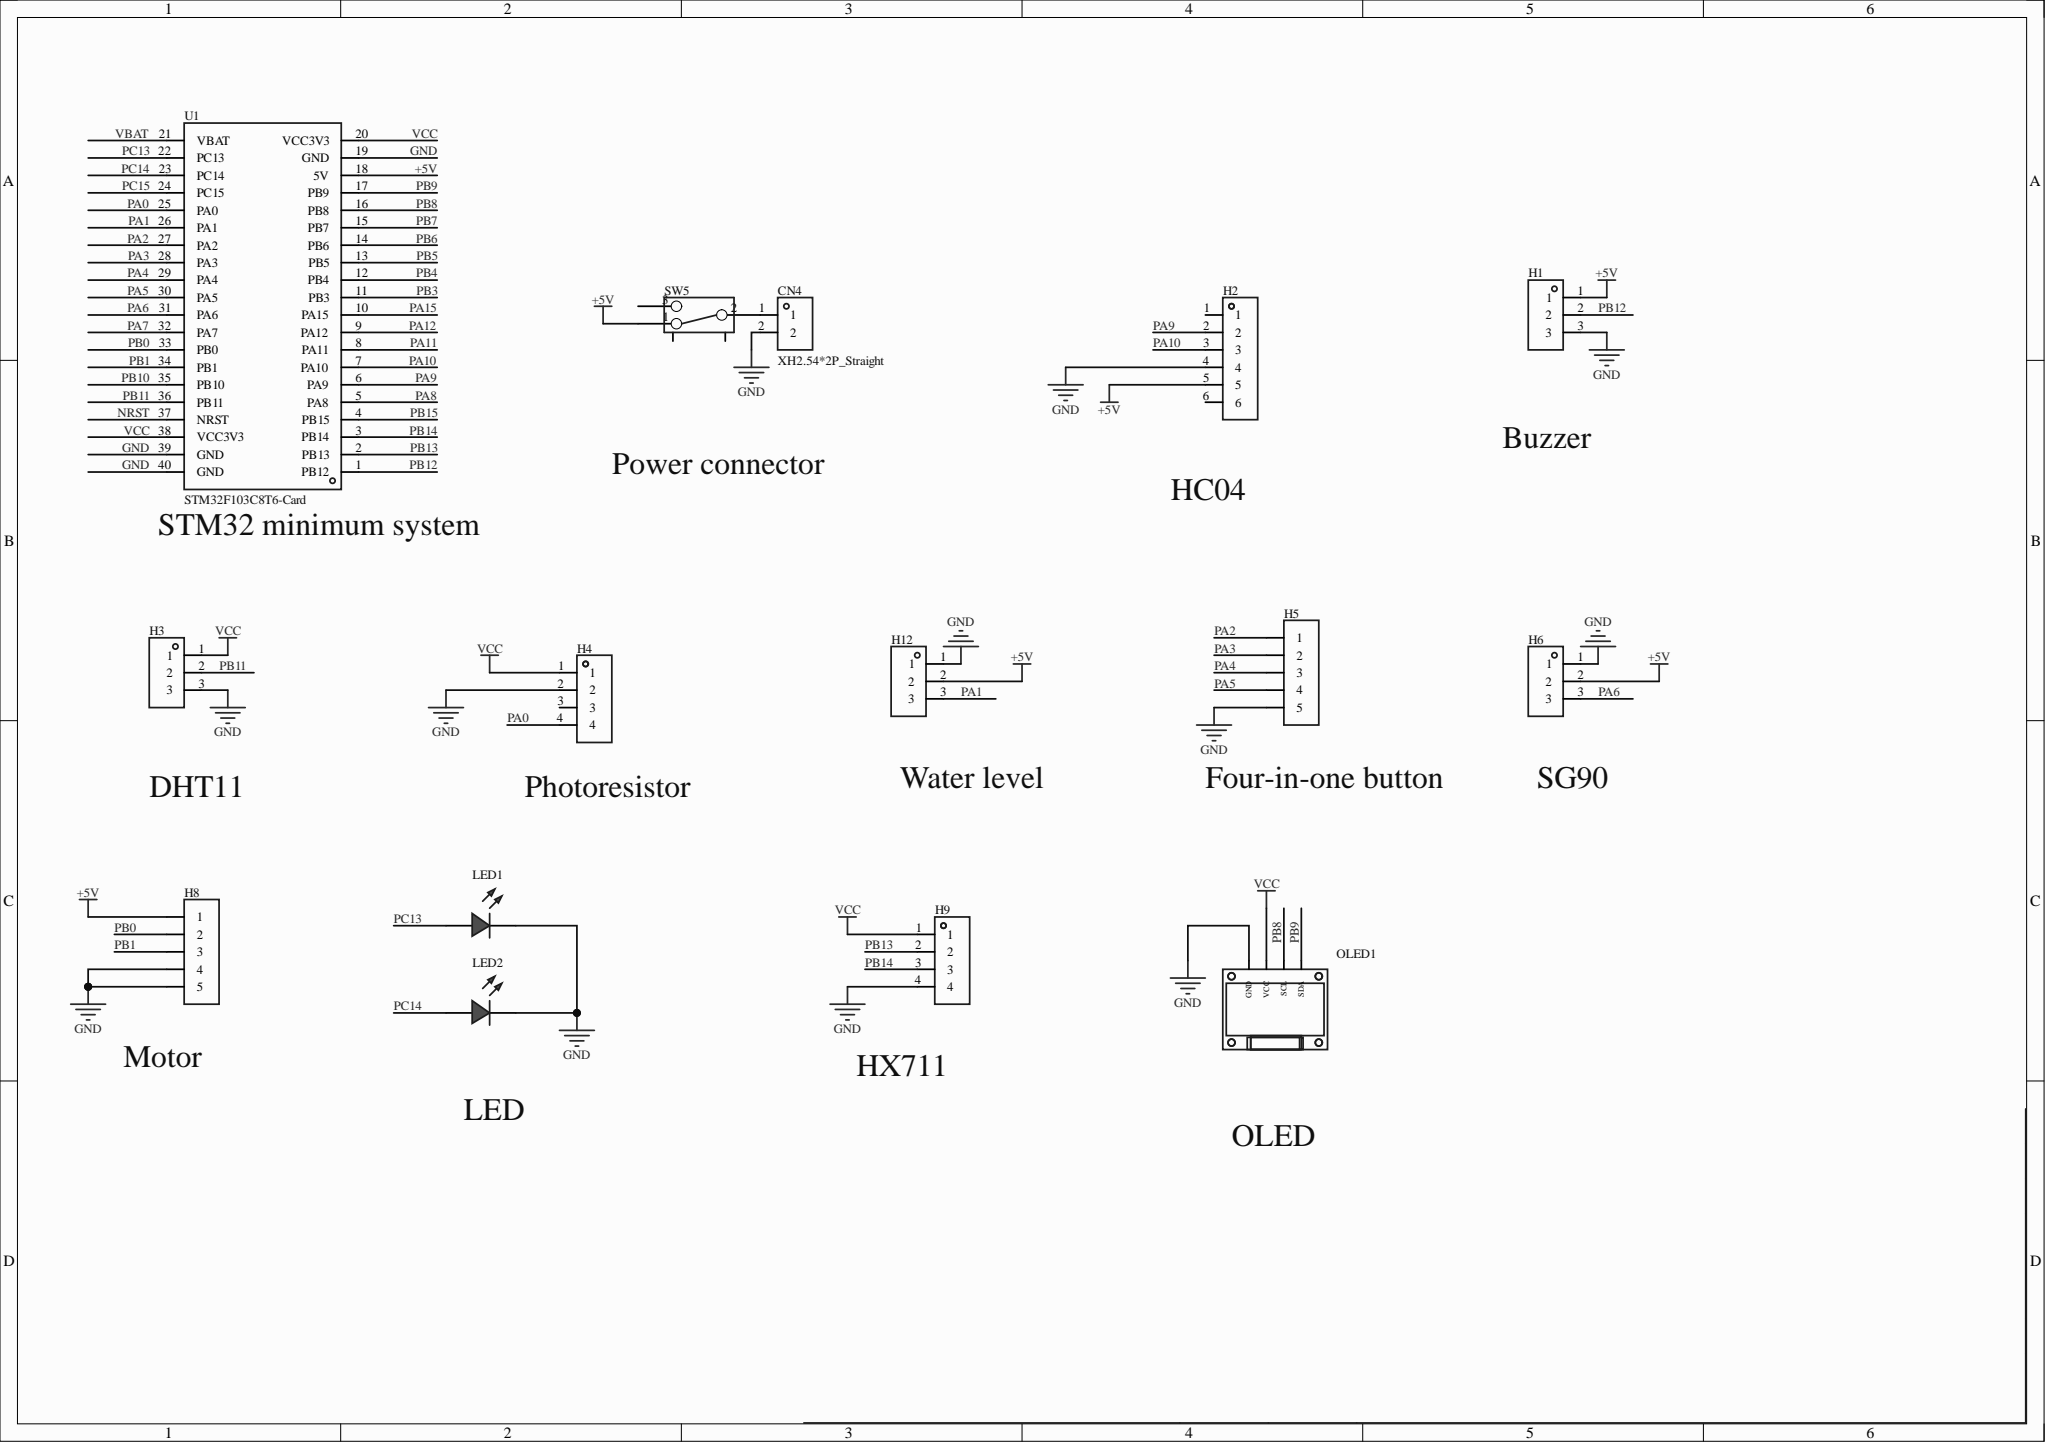Circuit board | Altium Designer | 15 parts | 23 nets
Bill of materials:
Comment,Description,Designator,Footprint,LibRef,Quantity
"XH2.54*2P_Straight","","CN4","CONN-TH_2P-P2.50-XH2.54-2P","XH2.54*2P_直插","1"
"","","H1, H3, H6, H12","HDR-TH_3P-P2.54-V-F","HDR-F_2.54_1x3P","4"
"","","H2","HDR-TH_6P-P2.54-V-F","HDR-F_2.54_1x6P","1"
"","","H4, H9","HDR-TH_4P-P2.54-V-F","HDR-F_2.54_1x4P","2"
"","","H5, H8","HDR-TH_5P-P2.54-V-F","HDR-F_2.54_1x5P","2"
"","","LED1, LED2","LED-TH_5mm","LED_TH-R_5mm","2"
"","","OLED1","0.96OLED_4P","0.96OLED模块_4P","1"
"","","SW5","拨动开关","拨动开关_正","1"
"STM32F103C8T6-Card","","U1","CONN-TH_L53.3-W22.9_STM32F103C8T6-CARD","STM32F103C8T6-Card","1"
Netlist (Protel format):
[
CN4
CONN-TH_2P-P2.50-XH2.54-2P
XH2.54*2P_Straight



]
[
H1
HDR-TH_3P-P2.54-V-F




]
[
H2
HDR-TH_6P-P2.54-V-F




]
[
H3
HDR-TH_3P-P2.54-V-F




]
[
H4
HDR-TH_4P-P2.54-V-F




]
[
H5
HDR-TH_5P-P2.54-V-F




]
[
H6
HDR-TH_3P-P2.54-V-F




]
[
H8
HDR-TH_5P-P2.54-V-F




]
[
H9
HDR-TH_4P-P2.54-V-F




]
[
H12
HDR-TH_3P-P2.54-V-F




]
[
LED1
LED-TH_5mm




]
[
LED2
LED-TH_5mm




]
[
OLED1
0.96OLED_4P




]
[
SW5
拨动开关




]
[
U1
CONN-TH_L53.3-W22.9_STM32F103C8T6-CARD
STM32F103C8T6-Card



]
(
VCC
H3-1
H4-1
H9-1
OLED1-2
U1-20
U1-38
)
(
PC14
LED2-1
U1-23
)
(
PC13
LED1-1
U1-22
)
(
PB14
H9-3
U1-3
)
(
PB13
H9-2
U1-2
)
(
PB12
H1-2
U1-1
)
(
PB11
H3-2
U1-36
)
(
PB9
OLED1-4
U1-17
)
(
PB8
OLED1-3
U1-16
)
(
PB1
H8-3
U1-34
)
(
PB0
H8-2
U1-33
)
(
PA10
H2-3
U1-7
)
(
PA9
H2-2
U1-6
)
(
PA6
H6-3
U1-31
)
(
PA5
H5-4
U1-30
)
(
PA4
H5-3
U1-29
)
(
PA3
H5-2
U1-28
)
(
PA2
H5-1
U1-27
)
(
PA1
H12-3
U1-26
)
(
PA0
H4-4
U1-25
)
(
NetCN4_1
CN4-1
SW5-2
)
(
GND
CN4-2
H1-3
H2-4
H3-3
H4-2
H5-5
H6-1
H8-4
H8-5
H9-4
H12-1
LED1-2
LED2-2
OLED1-1
U1-19
U1-39
U1-40
)
(
+5V
H1-1
H2-5
H6-2
H8-1
H12-2
SW5-1
U1-18
)